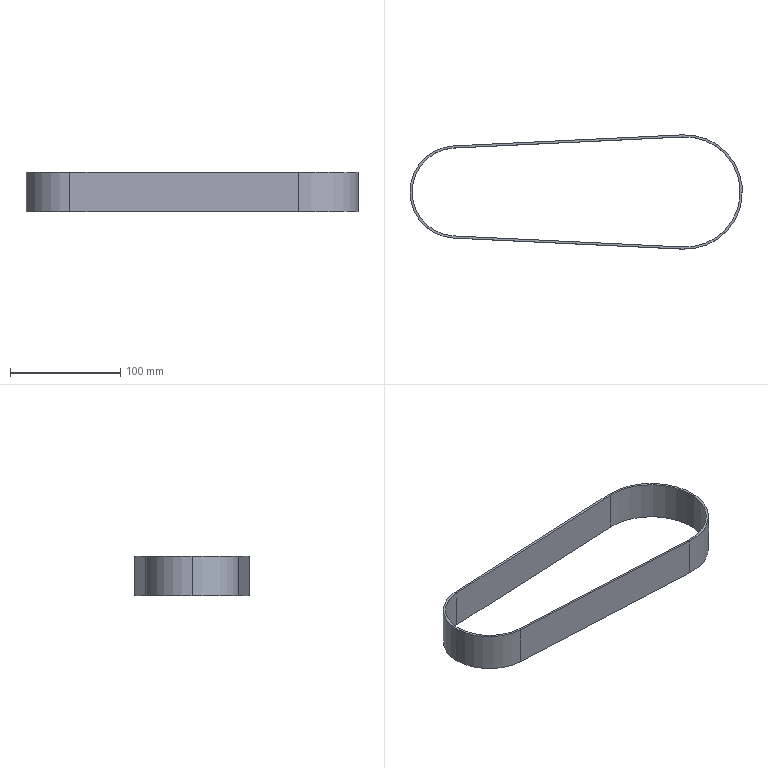Part | SolidWorks | features Extrusion 1 | 1 solid | 12 faces | box 301.927 x 103.927 x 35.6 mm | volume 49313 mm3 | cylinder 6 | plane 6 | commonest cylinder face diameters 80 x2 83.927 x2 100 x1 103.927 x1
STEP:
#1=CARTESIAN_POINT('',(-1.923,39.954,35.6));
#2=VERTEX_POINT('',#1);
#3=CARTESIAN_POINT('',(-40.,0.,35.6));
#4=VERTEX_POINT('',#3);
#5=CARTESIAN_POINT('',(0.,0.,35.6));
#6=DIRECTION('',(0.,0.,1.));
#7=DIRECTION('',(1.,0.,0.));
#8=AXIS2_PLACEMENT_3D('',#5,#6,#7);
#9=CIRCLE('',#8,40.);
#10=EDGE_CURVE('',#2,#4,#9,.T.);
#11=ORIENTED_EDGE('',*,*,#10,.T.);
#12=CARTESIAN_POINT('',(-40.,0.,0.));
#13=VERTEX_POINT('',#12);
#14=CARTESIAN_POINT('',(-40.,0.,35.6));
#15=DIRECTION('',(0.,0.,-1.));
#16=VECTOR('',#15,1000.);
#17=LINE('',#14,#16);
#18=EDGE_CURVE('',#4,#13,#17,.T.);
#19=ORIENTED_EDGE('',*,*,#18,.T.);
#20=CARTESIAN_POINT('',(-1.923,39.954,0.));
#21=VERTEX_POINT('',#20);
#22=CARTESIAN_POINT('',(0.,0.,0.));
#23=DIRECTION('',(0.,0.,1.));
#24=DIRECTION('',(1.,0.,0.));
#25=AXIS2_PLACEMENT_3D('',#22,#23,#24);
#26=CIRCLE('',#25,40.);
#27=EDGE_CURVE('',#21,#13,#26,.T.);
#28=ORIENTED_EDGE('',*,*,#27,.F.);
#29=CARTESIAN_POINT('',(-1.923,39.954,35.6));
#30=DIRECTION('',(0.,0.,-1.));
#31=VECTOR('',#30,1000.);
#32=LINE('',#29,#31);
#33=EDGE_CURVE('',#2,#21,#32,.T.);
#34=ORIENTED_EDGE('',*,*,#33,.F.);
#35=EDGE_LOOP('',(#11,#19,#28,#34));
#36=FACE_OUTER_BOUND('',#35,.T.);
#37=CARTESIAN_POINT('',(0.,0.,35.6));
#38=DIRECTION('',(0.,0.,-1.));
#39=DIRECTION('',(-1.,0.,0.));
#40=AXIS2_PLACEMENT_3D('',#37,#38,#39);
#41=CYLINDRICAL_SURFACE('',#40,40.);
#42=ADVANCED_FACE('',(#36),#41,.F.);
#43=CARTESIAN_POINT('',(-41.964,0.,35.6));
#44=VERTEX_POINT('',#43);
#45=CARTESIAN_POINT('',(-2.017,-41.915,35.6));
#46=VERTEX_POINT('',#45);
#47=CARTESIAN_POINT('',(0.,0.,35.6));
#48=DIRECTION('',(0.,0.,1.));
#49=DIRECTION('',(1.,0.,0.));
#50=AXIS2_PLACEMENT_3D('',#47,#48,#49);
#51=CIRCLE('',#50,41.964);
#52=EDGE_CURVE('',#44,#46,#51,.T.);
#53=ORIENTED_EDGE('',*,*,#52,.F.);
#54=CARTESIAN_POINT('',(-41.964,0.,0.));
#55=VERTEX_POINT('',#54);
#56=CARTESIAN_POINT('',(-41.964,0.,35.6));
#57=DIRECTION('',(0.,0.,-1.));
#58=VECTOR('',#57,1000.);
#59=LINE('',#56,#58);
#60=EDGE_CURVE('',#44,#55,#59,.T.);
#61=ORIENTED_EDGE('',*,*,#60,.T.);
#62=CARTESIAN_POINT('',(-2.017,-41.915,0.));
#63=VERTEX_POINT('',#62);
#64=CARTESIAN_POINT('',(0.,0.,0.));
#65=DIRECTION('',(0.,0.,1.));
#66=DIRECTION('',(1.,0.,0.));
#67=AXIS2_PLACEMENT_3D('',#64,#65,#66);
#68=CIRCLE('',#67,41.964);
#69=EDGE_CURVE('',#55,#63,#68,.T.);
#70=ORIENTED_EDGE('',*,*,#69,.T.);
#71=CARTESIAN_POINT('',(-2.017,-41.915,35.6));
#72=DIRECTION('',(0.,0.,-1.));
#73=VECTOR('',#72,1000.);
#74=LINE('',#71,#73);
#75=EDGE_CURVE('',#46,#63,#74,.T.);
#76=ORIENTED_EDGE('',*,*,#75,.F.);
#77=EDGE_LOOP('',(#53,#61,#70,#76));
#78=FACE_OUTER_BOUND('',#77,.T.);
#79=CARTESIAN_POINT('',(0.,0.,35.6));
#80=DIRECTION('',(0.,0.,-1.));
#81=DIRECTION('',(-1.,0.,0.));
#82=AXIS2_PLACEMENT_3D('',#79,#80,#81);
#83=CYLINDRICAL_SURFACE('',#82,41.964);
#84=ADVANCED_FACE('',(#78),#83,.T.);
#85=CARTESIAN_POINT('',(-2.017,41.915,35.6));
#86=VERTEX_POINT('',#85);
#87=CARTESIAN_POINT('',(0.,0.,35.6));
#88=DIRECTION('',(0.,0.,1.));
#89=DIRECTION('',(1.,0.,0.));
#90=AXIS2_PLACEMENT_3D('',#87,#88,#89);
#91=CIRCLE('',#90,41.964);
#92=EDGE_CURVE('',#86,#44,#91,.T.);
#93=ORIENTED_EDGE('',*,*,#92,.T.);
#94=ORIENTED_EDGE('',*,*,#52,.T.);
#95=CARTESIAN_POINT('',(205.502,-51.904,35.6));
#96=VERTEX_POINT('',#95);
#97=CARTESIAN_POINT('',(-2.017,-41.915,35.6));
#98=DIRECTION('',(0.9988,-0.04808,0.));
#99=VECTOR('',#98,1000.);
#100=LINE('',#97,#99);
#101=EDGE_CURVE('',#46,#96,#100,.T.);
#102=ORIENTED_EDGE('',*,*,#101,.T.);
#103=CARTESIAN_POINT('',(205.502,51.904,35.6));
#104=VERTEX_POINT('',#103);
#105=CARTESIAN_POINT('',(208.,0.,35.6));
#106=DIRECTION('',(0.,0.,1.));
#107=DIRECTION('',(1.,0.,0.));
#108=AXIS2_PLACEMENT_3D('',#105,#106,#107);
#109=CIRCLE('',#108,51.964);
#110=EDGE_CURVE('',#96,#104,#109,.T.);
#111=ORIENTED_EDGE('',*,*,#110,.T.);
#112=CARTESIAN_POINT('',(-2.017,41.915,35.6));
#113=DIRECTION('',(-0.9988,-0.04808,0.));
#114=VECTOR('',#113,1000.);
#115=LINE('',#112,#114);
#116=EDGE_CURVE('',#104,#86,#115,.T.);
#117=ORIENTED_EDGE('',*,*,#116,.T.);
#118=EDGE_LOOP('',(#93,#94,#102,#111,#117));
#119=FACE_OUTER_BOUND('',#118,.T.);
#120=CARTESIAN_POINT('',(-1.923,-39.954,35.6));
#121=VERTEX_POINT('',#120);
#122=CARTESIAN_POINT('',(205.596,-49.942,35.6));
#123=VERTEX_POINT('',#122);
#124=CARTESIAN_POINT('',(-1.923,-39.954,35.6));
#125=DIRECTION('',(0.9988,-0.04808,0.));
#126=VECTOR('',#125,1000.);
#127=LINE('',#124,#126);
#128=EDGE_CURVE('',#121,#123,#127,.T.);
#129=ORIENTED_EDGE('',*,*,#128,.F.);
#130=CARTESIAN_POINT('',(0.,0.,35.6));
#131=DIRECTION('',(0.,0.,1.));
#132=DIRECTION('',(1.,0.,0.));
#133=AXIS2_PLACEMENT_3D('',#130,#131,#132);
#134=CIRCLE('',#133,40.);
#135=EDGE_CURVE('',#4,#121,#134,.T.);
#136=ORIENTED_EDGE('',*,*,#135,.F.);
#137=ORIENTED_EDGE('',*,*,#10,.F.);
#138=CARTESIAN_POINT('',(205.596,49.942,35.6));
#139=VERTEX_POINT('',#138);
#140=CARTESIAN_POINT('',(-1.923,39.954,35.6));
#141=DIRECTION('',(-0.9988,-0.04808,0.));
#142=VECTOR('',#141,1000.);
#143=LINE('',#140,#142);
#144=EDGE_CURVE('',#139,#2,#143,.T.);
#145=ORIENTED_EDGE('',*,*,#144,.F.);
#146=CARTESIAN_POINT('',(208.,0.,35.6));
#147=DIRECTION('',(0.,0.,1.));
#148=DIRECTION('',(1.,0.,0.));
#149=AXIS2_PLACEMENT_3D('',#146,#147,#148);
#150=CIRCLE('',#149,50.);
#151=EDGE_CURVE('',#123,#139,#150,.T.);
#152=ORIENTED_EDGE('',*,*,#151,.F.);
#153=EDGE_LOOP('',(#129,#136,#137,#145,#152));
#154=FACE_BOUND('',#153,.T.);
#155=CARTESIAN_POINT('',(0.,0.,35.6));
#156=DIRECTION('',(0.,0.,1.));
#157=DIRECTION('',(1.,0.,0.));
#158=AXIS2_PLACEMENT_3D('',#155,#156,#157);
#159=PLANE('',#158);
#160=ADVANCED_FACE('',(#119,#154),#159,.T.);
#161=CARTESIAN_POINT('',(-2.017,41.915,0.));
#162=VERTEX_POINT('',#161);
#163=CARTESIAN_POINT('',(0.,0.,0.));
#164=DIRECTION('',(0.,0.,1.));
#165=DIRECTION('',(1.,0.,0.));
#166=AXIS2_PLACEMENT_3D('',#163,#164,#165);
#167=CIRCLE('',#166,41.964);
#168=EDGE_CURVE('',#162,#55,#167,.T.);
#169=ORIENTED_EDGE('',*,*,#168,.F.);
#170=CARTESIAN_POINT('',(205.502,51.904,0.));
#171=VERTEX_POINT('',#170);
#172=CARTESIAN_POINT('',(-2.017,41.915,0.));
#173=DIRECTION('',(-0.9988,-0.04808,0.));
#174=VECTOR('',#173,1000.);
#175=LINE('',#172,#174);
#176=EDGE_CURVE('',#171,#162,#175,.T.);
#177=ORIENTED_EDGE('',*,*,#176,.F.);
#178=CARTESIAN_POINT('',(205.502,-51.904,0.));
#179=VERTEX_POINT('',#178);
#180=CARTESIAN_POINT('',(208.,0.,0.));
#181=DIRECTION('',(0.,0.,1.));
#182=DIRECTION('',(1.,0.,0.));
#183=AXIS2_PLACEMENT_3D('',#180,#181,#182);
#184=CIRCLE('',#183,51.964);
#185=EDGE_CURVE('',#179,#171,#184,.T.);
#186=ORIENTED_EDGE('',*,*,#185,.F.);
#187=CARTESIAN_POINT('',(-2.017,-41.915,0.));
#188=DIRECTION('',(0.9988,-0.04808,0.));
#189=VECTOR('',#188,1000.);
#190=LINE('',#187,#189);
#191=EDGE_CURVE('',#63,#179,#190,.T.);
#192=ORIENTED_EDGE('',*,*,#191,.F.);
#193=ORIENTED_EDGE('',*,*,#69,.F.);
#194=EDGE_LOOP('',(#169,#177,#186,#192,#193));
#195=FACE_OUTER_BOUND('',#194,.T.);
#196=ORIENTED_EDGE('',*,*,#27,.T.);
#197=CARTESIAN_POINT('',(-1.923,-39.954,0.));
#198=VERTEX_POINT('',#197);
#199=CARTESIAN_POINT('',(0.,0.,0.));
#200=DIRECTION('',(0.,0.,1.));
#201=DIRECTION('',(1.,0.,0.));
#202=AXIS2_PLACEMENT_3D('',#199,#200,#201);
#203=CIRCLE('',#202,40.);
#204=EDGE_CURVE('',#13,#198,#203,.T.);
#205=ORIENTED_EDGE('',*,*,#204,.T.);
#206=CARTESIAN_POINT('',(205.596,-49.942,0.));
#207=VERTEX_POINT('',#206);
#208=CARTESIAN_POINT('',(-1.923,-39.954,0.));
#209=DIRECTION('',(0.9988,-0.04808,0.));
#210=VECTOR('',#209,1000.);
#211=LINE('',#208,#210);
#212=EDGE_CURVE('',#198,#207,#211,.T.);
#213=ORIENTED_EDGE('',*,*,#212,.T.);
#214=CARTESIAN_POINT('',(205.596,49.942,0.));
#215=VERTEX_POINT('',#214);
#216=CARTESIAN_POINT('',(208.,0.,0.));
#217=DIRECTION('',(0.,0.,1.));
#218=DIRECTION('',(1.,0.,0.));
#219=AXIS2_PLACEMENT_3D('',#216,#217,#218);
#220=CIRCLE('',#219,50.);
#221=EDGE_CURVE('',#207,#215,#220,.T.);
#222=ORIENTED_EDGE('',*,*,#221,.T.);
#223=CARTESIAN_POINT('',(-1.923,39.954,0.));
#224=DIRECTION('',(-0.9988,-0.04808,0.));
#225=VECTOR('',#224,1000.);
#226=LINE('',#223,#225);
#227=EDGE_CURVE('',#215,#21,#226,.T.);
#228=ORIENTED_EDGE('',*,*,#227,.T.);
#229=EDGE_LOOP('',(#196,#205,#213,#222,#228));
#230=FACE_BOUND('',#229,.T.);
#231=CARTESIAN_POINT('',(0.,0.,0.));
#232=DIRECTION('',(0.,0.,1.));
#233=DIRECTION('',(1.,0.,0.));
#234=AXIS2_PLACEMENT_3D('',#231,#232,#233);
#235=PLANE('',#234);
#236=ADVANCED_FACE('',(#195,#230),#235,.F.);
#237=ORIENTED_EDGE('',*,*,#60,.F.);
#238=ORIENTED_EDGE('',*,*,#92,.F.);
#239=CARTESIAN_POINT('',(-2.017,41.915,35.6));
#240=DIRECTION('',(0.,0.,-1.));
#241=VECTOR('',#240,1000.);
#242=LINE('',#239,#241);
#243=EDGE_CURVE('',#86,#162,#242,.T.);
#244=ORIENTED_EDGE('',*,*,#243,.T.);
#245=ORIENTED_EDGE('',*,*,#168,.T.);
#246=EDGE_LOOP('',(#237,#238,#244,#245));
#247=FACE_OUTER_BOUND('',#246,.T.);
#248=CARTESIAN_POINT('',(0.,0.,35.6));
#249=DIRECTION('',(0.,0.,-1.));
#250=DIRECTION('',(-1.,0.,0.));
#251=AXIS2_PLACEMENT_3D('',#248,#249,#250);
#252=CYLINDRICAL_SURFACE('',#251,41.964);
#253=ADVANCED_FACE('',(#247),#252,.T.);
#254=ORIENTED_EDGE('',*,*,#191,.T.);
#255=CARTESIAN_POINT('',(205.502,-51.904,35.6));
#256=DIRECTION('',(0.,0.,-1.));
#257=VECTOR('',#256,1000.);
#258=LINE('',#255,#257);
#259=EDGE_CURVE('',#96,#179,#258,.T.);
#260=ORIENTED_EDGE('',*,*,#259,.F.);
#261=ORIENTED_EDGE('',*,*,#101,.F.);
#262=ORIENTED_EDGE('',*,*,#75,.T.);
#263=EDGE_LOOP('',(#254,#260,#261,#262));
#264=FACE_OUTER_BOUND('',#263,.T.);
#265=CARTESIAN_POINT('',(-2.017,-41.915,35.6));
#266=DIRECTION('',(0.04808,0.9988,0.));
#267=DIRECTION('',(-0.9988,0.04808,0.));
#268=AXIS2_PLACEMENT_3D('',#265,#266,#267);
#269=PLANE('',#268);
#270=ADVANCED_FACE('',(#264),#269,.F.);
#271=ORIENTED_EDGE('',*,*,#185,.T.);
#272=CARTESIAN_POINT('',(205.502,51.904,35.6));
#273=DIRECTION('',(0.,0.,-1.));
#274=VECTOR('',#273,1000.);
#275=LINE('',#272,#274);
#276=EDGE_CURVE('',#104,#171,#275,.T.);
#277=ORIENTED_EDGE('',*,*,#276,.F.);
#278=ORIENTED_EDGE('',*,*,#110,.F.);
#279=ORIENTED_EDGE('',*,*,#259,.T.);
#280=EDGE_LOOP('',(#271,#277,#278,#279));
#281=FACE_OUTER_BOUND('',#280,.T.);
#282=CARTESIAN_POINT('',(208.,0.,35.6));
#283=DIRECTION('',(0.,0.,-1.));
#284=DIRECTION('',(-1.,0.,0.));
#285=AXIS2_PLACEMENT_3D('',#282,#283,#284);
#286=CYLINDRICAL_SURFACE('',#285,51.964);
#287=ADVANCED_FACE('',(#281),#286,.T.);
#288=ORIENTED_EDGE('',*,*,#176,.T.);
#289=ORIENTED_EDGE('',*,*,#243,.F.);
#290=ORIENTED_EDGE('',*,*,#116,.F.);
#291=ORIENTED_EDGE('',*,*,#276,.T.);
#292=EDGE_LOOP('',(#288,#289,#290,#291));
#293=FACE_OUTER_BOUND('',#292,.T.);
#294=CARTESIAN_POINT('',(-2.017,41.915,35.6));
#295=DIRECTION('',(0.04808,-0.9988,0.));
#296=DIRECTION('',(0.9988,0.04808,0.));
#297=AXIS2_PLACEMENT_3D('',#294,#295,#296);
#298=PLANE('',#297);
#299=ADVANCED_FACE('',(#293),#298,.F.);
#300=ORIENTED_EDGE('',*,*,#18,.F.);
#301=ORIENTED_EDGE('',*,*,#135,.T.);
#302=CARTESIAN_POINT('',(-1.923,-39.954,35.6));
#303=DIRECTION('',(0.,0.,-1.));
#304=VECTOR('',#303,1000.);
#305=LINE('',#302,#304);
#306=EDGE_CURVE('',#121,#198,#305,.T.);
#307=ORIENTED_EDGE('',*,*,#306,.T.);
#308=ORIENTED_EDGE('',*,*,#204,.F.);
#309=EDGE_LOOP('',(#300,#301,#307,#308));
#310=FACE_OUTER_BOUND('',#309,.T.);
#311=CARTESIAN_POINT('',(0.,0.,35.6));
#312=DIRECTION('',(0.,0.,-1.));
#313=DIRECTION('',(-1.,0.,0.));
#314=AXIS2_PLACEMENT_3D('',#311,#312,#313);
#315=CYLINDRICAL_SURFACE('',#314,40.);
#316=ADVANCED_FACE('',(#310),#315,.F.);
#317=ORIENTED_EDGE('',*,*,#212,.F.);
#318=ORIENTED_EDGE('',*,*,#306,.F.);
#319=ORIENTED_EDGE('',*,*,#128,.T.);
#320=CARTESIAN_POINT('',(205.596,-49.942,35.6));
#321=DIRECTION('',(0.,0.,-1.));
#322=VECTOR('',#321,1000.);
#323=LINE('',#320,#322);
#324=EDGE_CURVE('',#123,#207,#323,.T.);
#325=ORIENTED_EDGE('',*,*,#324,.T.);
#326=EDGE_LOOP('',(#317,#318,#319,#325));
#327=FACE_OUTER_BOUND('',#326,.T.);
#328=CARTESIAN_POINT('',(-1.923,-39.954,35.6));
#329=DIRECTION('',(0.04808,0.9988,0.));
#330=DIRECTION('',(-0.9988,0.04808,0.));
#331=AXIS2_PLACEMENT_3D('',#328,#329,#330);
#332=PLANE('',#331);
#333=ADVANCED_FACE('',(#327),#332,.T.);
#334=ORIENTED_EDGE('',*,*,#221,.F.);
#335=ORIENTED_EDGE('',*,*,#324,.F.);
#336=ORIENTED_EDGE('',*,*,#151,.T.);
#337=CARTESIAN_POINT('',(205.596,49.942,35.6));
#338=DIRECTION('',(0.,0.,-1.));
#339=VECTOR('',#338,1000.);
#340=LINE('',#337,#339);
#341=EDGE_CURVE('',#139,#215,#340,.T.);
#342=ORIENTED_EDGE('',*,*,#341,.T.);
#343=EDGE_LOOP('',(#334,#335,#336,#342));
#344=FACE_OUTER_BOUND('',#343,.T.);
#345=CARTESIAN_POINT('',(208.,0.,35.6));
#346=DIRECTION('',(0.,0.,-1.));
#347=DIRECTION('',(-1.,0.,0.));
#348=AXIS2_PLACEMENT_3D('',#345,#346,#347);
#349=CYLINDRICAL_SURFACE('',#348,50.);
#350=ADVANCED_FACE('',(#344),#349,.F.);
#351=ORIENTED_EDGE('',*,*,#227,.F.);
#352=ORIENTED_EDGE('',*,*,#341,.F.);
#353=ORIENTED_EDGE('',*,*,#144,.T.);
#354=ORIENTED_EDGE('',*,*,#33,.T.);
#355=EDGE_LOOP('',(#351,#352,#353,#354));
#356=FACE_OUTER_BOUND('',#355,.T.);
#357=CARTESIAN_POINT('',(-1.923,39.954,35.6));
#358=DIRECTION('',(0.04808,-0.9988,0.));
#359=DIRECTION('',(0.9988,0.04808,0.));
#360=AXIS2_PLACEMENT_3D('',#357,#358,#359);
#361=PLANE('',#360);
#362=ADVANCED_FACE('',(#356),#361,.T.);
#363=CLOSED_SHELL('',(#42,#84,#160,#236,#253,#270,#287,#299,#316,#333,#350,#362));
#364=MANIFOLD_SOLID_BREP('',#363);
#365=CARTESIAN_POINT('',(0.,0.,0.));
#366=DIRECTION('',(0.,0.,1.));
#367=DIRECTION('',(1.,0.,0.));
#368=AXIS2_PLACEMENT_3D('',#365,#366,#367);
#369=(LENGTH_UNIT()NAMED_UNIT(*)SI_UNIT(.MILLI.,.METRE.));
#370=UNCERTAINTY_MEASURE_WITH_UNIT(LENGTH_MEASURE(0.00001),#369,'','');
#371=(NAMED_UNIT(*)PLANE_ANGLE_UNIT()SI_UNIT($,.RADIAN.));
#372=(NAMED_UNIT(*)SI_UNIT($,.STERADIAN.)SOLID_ANGLE_UNIT());
#373=(GEOMETRIC_REPRESENTATION_CONTEXT(3)GLOBAL_UNCERTAINTY_ASSIGNED_CONTEXT((#370))GLOBAL_UNIT_ASSIGNED_CONTEXT((#369,#371,#372))REPRESENTATION_CONTEXT('',''));
#374=ADVANCED_BREP_SHAPE_REPRESENTATION('',(#364,#368),#373);